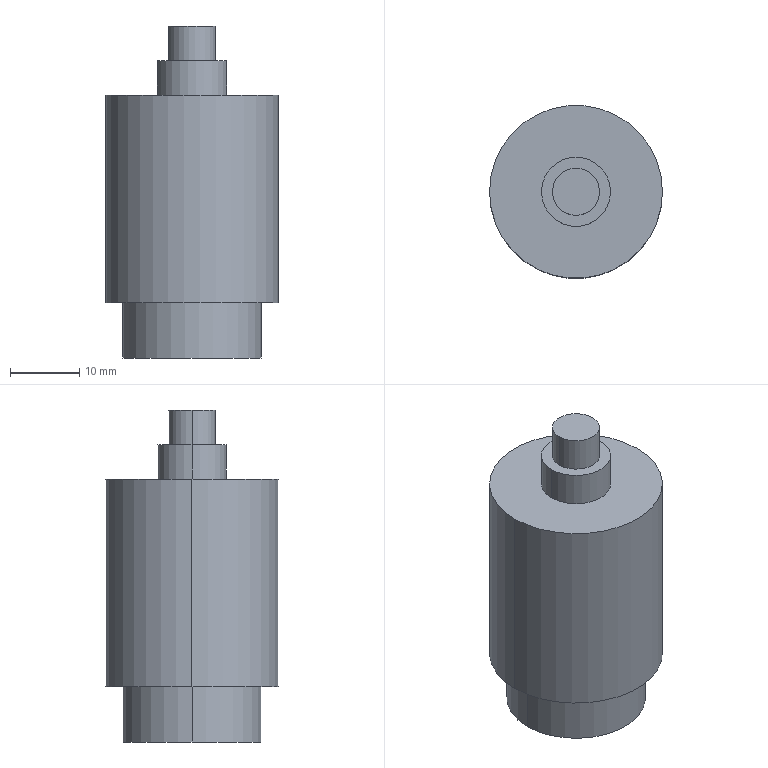Part | SolidWorks | features ICE 3, Extrusion 1 | 1 solid | 13 faces | box 25 x 25 x 48 mm | volume 17814 mm3 | cylinder 8 | plane 5 | commonest cylinder face diameters 6.8 x2 10 x2 20 x2 25 x2
STEP:
#1=CARTESIAN_POINT('',(-10.,0.,-38.));
#2=VERTEX_POINT('',#1);
#3=CARTESIAN_POINT('',(10.,0.,-38.));
#4=VERTEX_POINT('',#3);
#5=CARTESIAN_POINT('',(0.,0.,-38.));
#6=DIRECTION('',(0.,0.,-1.));
#7=DIRECTION('',(-1.,0.,0.));
#8=AXIS2_PLACEMENT_3D('',#5,#6,#7);
#9=CIRCLE('',#8,10.);
#10=EDGE_CURVE('',#2,#4,#9,.T.);
#11=ORIENTED_EDGE('',*,*,#10,.F.);
#12=CARTESIAN_POINT('',(-10.,0.,-30.));
#13=VERTEX_POINT('',#12);
#14=CARTESIAN_POINT('',(-10.,0.,-38.));
#15=DIRECTION('',(0.,0.,1.));
#16=VECTOR('',#15,1000.);
#17=LINE('',#14,#16);
#18=EDGE_CURVE('',#2,#13,#17,.T.);
#19=ORIENTED_EDGE('',*,*,#18,.T.);
#20=CARTESIAN_POINT('',(10.,0.,-30.));
#21=VERTEX_POINT('',#20);
#22=CARTESIAN_POINT('',(0.,0.,-30.));
#23=DIRECTION('',(0.,0.,-1.));
#24=DIRECTION('',(-1.,0.,0.));
#25=AXIS2_PLACEMENT_3D('',#22,#23,#24);
#26=CIRCLE('',#25,10.);
#27=EDGE_CURVE('',#13,#21,#26,.T.);
#28=ORIENTED_EDGE('',*,*,#27,.T.);
#29=CARTESIAN_POINT('',(10.,0.,-38.));
#30=DIRECTION('',(0.,0.,1.));
#31=VECTOR('',#30,1000.);
#32=LINE('',#29,#31);
#33=EDGE_CURVE('',#4,#21,#32,.T.);
#34=ORIENTED_EDGE('',*,*,#33,.F.);
#35=EDGE_LOOP('',(#11,#19,#28,#34));
#36=FACE_OUTER_BOUND('',#35,.T.);
#37=CARTESIAN_POINT('',(0.,0.,-38.));
#38=DIRECTION('',(0.,0.,1.));
#39=DIRECTION('',(1.,0.,0.));
#40=AXIS2_PLACEMENT_3D('',#37,#38,#39);
#41=CYLINDRICAL_SURFACE('',#40,10.);
#42=ADVANCED_FACE('',(#36),#41,.T.);
#43=CARTESIAN_POINT('',(-12.5,0.,-30.));
#44=VERTEX_POINT('',#43);
#45=CARTESIAN_POINT('',(12.5,0.,-30.));
#46=VERTEX_POINT('',#45);
#47=CARTESIAN_POINT('',(0.,0.,-30.));
#48=DIRECTION('',(0.,0.,-1.));
#49=DIRECTION('',(-1.,0.,0.));
#50=AXIS2_PLACEMENT_3D('',#47,#48,#49);
#51=CIRCLE('',#50,12.5);
#52=EDGE_CURVE('',#44,#46,#51,.T.);
#53=ORIENTED_EDGE('',*,*,#52,.F.);
#54=CARTESIAN_POINT('',(-12.5,0.,0.));
#55=VERTEX_POINT('',#54);
#56=CARTESIAN_POINT('',(-12.5,0.,-30.));
#57=DIRECTION('',(0.,0.,1.));
#58=VECTOR('',#57,1000.);
#59=LINE('',#56,#58);
#60=EDGE_CURVE('',#44,#55,#59,.T.);
#61=ORIENTED_EDGE('',*,*,#60,.T.);
#62=CARTESIAN_POINT('',(12.5,0.,0.));
#63=VERTEX_POINT('',#62);
#64=CARTESIAN_POINT('',(0.,0.,0.));
#65=DIRECTION('',(0.,0.,-1.));
#66=DIRECTION('',(-1.,0.,0.));
#67=AXIS2_PLACEMENT_3D('',#64,#65,#66);
#68=CIRCLE('',#67,12.5);
#69=EDGE_CURVE('',#55,#63,#68,.T.);
#70=ORIENTED_EDGE('',*,*,#69,.T.);
#71=CARTESIAN_POINT('',(12.5,0.,-30.));
#72=DIRECTION('',(0.,0.,1.));
#73=VECTOR('',#72,1000.);
#74=LINE('',#71,#73);
#75=EDGE_CURVE('',#46,#63,#74,.T.);
#76=ORIENTED_EDGE('',*,*,#75,.F.);
#77=EDGE_LOOP('',(#53,#61,#70,#76));
#78=FACE_OUTER_BOUND('',#77,.T.);
#79=CARTESIAN_POINT('',(0.,0.,-30.));
#80=DIRECTION('',(0.,0.,1.));
#81=DIRECTION('',(1.,0.,0.));
#82=AXIS2_PLACEMENT_3D('',#79,#80,#81);
#83=CYLINDRICAL_SURFACE('',#82,12.5);
#84=ADVANCED_FACE('',(#78),#83,.T.);
#85=CARTESIAN_POINT('',(3.4,0.,10.));
#86=VERTEX_POINT('',#85);
#87=CARTESIAN_POINT('',(-3.4,0.,10.));
#88=VERTEX_POINT('',#87);
#89=CARTESIAN_POINT('',(0.,0.,10.));
#90=DIRECTION('',(0.,0.,1.));
#91=DIRECTION('',(1.,0.,0.));
#92=AXIS2_PLACEMENT_3D('',#89,#90,#91);
#93=CIRCLE('',#92,3.4);
#94=EDGE_CURVE('',#86,#88,#93,.T.);
#95=ORIENTED_EDGE('',*,*,#94,.F.);
#96=CARTESIAN_POINT('',(3.4,0.,5.));
#97=VERTEX_POINT('',#96);
#98=CARTESIAN_POINT('',(3.4,0.,10.));
#99=DIRECTION('',(0.,0.,-1.));
#100=VECTOR('',#99,1000.);
#101=LINE('',#98,#100);
#102=EDGE_CURVE('',#86,#97,#101,.T.);
#103=ORIENTED_EDGE('',*,*,#102,.T.);
#104=CARTESIAN_POINT('',(-3.4,0.,5.));
#105=VERTEX_POINT('',#104);
#106=CARTESIAN_POINT('',(0.,0.,5.));
#107=DIRECTION('',(0.,0.,1.));
#108=DIRECTION('',(1.,0.,0.));
#109=AXIS2_PLACEMENT_3D('',#106,#107,#108);
#110=CIRCLE('',#109,3.4);
#111=EDGE_CURVE('',#97,#105,#110,.T.);
#112=ORIENTED_EDGE('',*,*,#111,.T.);
#113=CARTESIAN_POINT('',(-3.4,0.,10.));
#114=DIRECTION('',(0.,0.,-1.));
#115=VECTOR('',#114,1000.);
#116=LINE('',#113,#115);
#117=EDGE_CURVE('',#88,#105,#116,.T.);
#118=ORIENTED_EDGE('',*,*,#117,.F.);
#119=EDGE_LOOP('',(#95,#103,#112,#118));
#120=FACE_OUTER_BOUND('',#119,.T.);
#121=CARTESIAN_POINT('',(0.,0.,10.));
#122=DIRECTION('',(0.,0.,-1.));
#123=DIRECTION('',(-1.,0.,0.));
#124=AXIS2_PLACEMENT_3D('',#121,#122,#123);
#125=CYLINDRICAL_SURFACE('',#124,3.4);
#126=ADVANCED_FACE('',(#120),#125,.T.);
#127=CARTESIAN_POINT('',(5.,0.,5.));
#128=VERTEX_POINT('',#127);
#129=CARTESIAN_POINT('',(-5.,0.,5.));
#130=VERTEX_POINT('',#129);
#131=CARTESIAN_POINT('',(0.,0.,5.));
#132=DIRECTION('',(0.,0.,1.));
#133=DIRECTION('',(1.,0.,0.));
#134=AXIS2_PLACEMENT_3D('',#131,#132,#133);
#135=CIRCLE('',#134,5.);
#136=EDGE_CURVE('',#128,#130,#135,.T.);
#137=ORIENTED_EDGE('',*,*,#136,.F.);
#138=CARTESIAN_POINT('',(5.,0.,0.));
#139=VERTEX_POINT('',#138);
#140=CARTESIAN_POINT('',(5.,0.,5.));
#141=DIRECTION('',(0.,0.,-1.));
#142=VECTOR('',#141,1000.);
#143=LINE('',#140,#142);
#144=EDGE_CURVE('',#128,#139,#143,.T.);
#145=ORIENTED_EDGE('',*,*,#144,.T.);
#146=CARTESIAN_POINT('',(-5.,0.,0.));
#147=VERTEX_POINT('',#146);
#148=CARTESIAN_POINT('',(0.,0.,0.));
#149=DIRECTION('',(0.,0.,-1.));
#150=DIRECTION('',(-1.,0.,0.));
#151=AXIS2_PLACEMENT_3D('',#148,#149,#150);
#152=CIRCLE('',#151,5.);
#153=EDGE_CURVE('',#147,#139,#152,.T.);
#154=ORIENTED_EDGE('',*,*,#153,.F.);
#155=CARTESIAN_POINT('',(-5.,0.,5.));
#156=DIRECTION('',(0.,0.,-1.));
#157=VECTOR('',#156,1000.);
#158=LINE('',#155,#157);
#159=EDGE_CURVE('',#130,#147,#158,.T.);
#160=ORIENTED_EDGE('',*,*,#159,.F.);
#161=EDGE_LOOP('',(#137,#145,#154,#160));
#162=FACE_OUTER_BOUND('',#161,.T.);
#163=CARTESIAN_POINT('',(0.,0.,5.));
#164=DIRECTION('',(0.,0.,-1.));
#165=DIRECTION('',(-1.,0.,0.));
#166=AXIS2_PLACEMENT_3D('',#163,#164,#165);
#167=CYLINDRICAL_SURFACE('',#166,5.);
#168=ADVANCED_FACE('',(#162),#167,.T.);
#169=CARTESIAN_POINT('',(0.,0.,-30.));
#170=DIRECTION('',(0.,0.,-1.));
#171=DIRECTION('',(-1.,0.,0.));
#172=AXIS2_PLACEMENT_3D('',#169,#170,#171);
#173=CIRCLE('',#172,12.5);
#174=EDGE_CURVE('',#46,#44,#173,.T.);
#175=ORIENTED_EDGE('',*,*,#174,.T.);
#176=ORIENTED_EDGE('',*,*,#52,.T.);
#177=EDGE_LOOP('',(#175,#176));
#178=FACE_OUTER_BOUND('',#177,.T.);
#179=CARTESIAN_POINT('',(0.,0.,-30.));
#180=DIRECTION('',(0.,0.,-1.));
#181=DIRECTION('',(-1.,0.,0.));
#182=AXIS2_PLACEMENT_3D('',#179,#180,#181);
#183=CIRCLE('',#182,10.);
#184=EDGE_CURVE('',#21,#13,#183,.T.);
#185=ORIENTED_EDGE('',*,*,#184,.F.);
#186=ORIENTED_EDGE('',*,*,#27,.F.);
#187=EDGE_LOOP('',(#185,#186));
#188=FACE_BOUND('',#187,.T.);
#189=CARTESIAN_POINT('',(0.,0.,-30.));
#190=DIRECTION('',(0.,0.,-1.));
#191=DIRECTION('',(-1.,0.,0.));
#192=AXIS2_PLACEMENT_3D('',#189,#190,#191);
#193=PLANE('',#192);
#194=ADVANCED_FACE('',(#178,#188),#193,.T.);
#195=CARTESIAN_POINT('',(0.,0.,5.));
#196=DIRECTION('',(0.,0.,1.));
#197=DIRECTION('',(1.,0.,0.));
#198=AXIS2_PLACEMENT_3D('',#195,#196,#197);
#199=CIRCLE('',#198,5.);
#200=EDGE_CURVE('',#130,#128,#199,.T.);
#201=ORIENTED_EDGE('',*,*,#200,.T.);
#202=ORIENTED_EDGE('',*,*,#136,.T.);
#203=EDGE_LOOP('',(#201,#202));
#204=FACE_OUTER_BOUND('',#203,.T.);
#205=CARTESIAN_POINT('',(0.,0.,5.));
#206=DIRECTION('',(0.,0.,1.));
#207=DIRECTION('',(1.,0.,0.));
#208=AXIS2_PLACEMENT_3D('',#205,#206,#207);
#209=CIRCLE('',#208,3.4);
#210=EDGE_CURVE('',#105,#97,#209,.T.);
#211=ORIENTED_EDGE('',*,*,#210,.F.);
#212=ORIENTED_EDGE('',*,*,#111,.F.);
#213=EDGE_LOOP('',(#211,#212));
#214=FACE_BOUND('',#213,.T.);
#215=CARTESIAN_POINT('',(0.,0.,5.));
#216=DIRECTION('',(0.,0.,1.));
#217=DIRECTION('',(1.,0.,0.));
#218=AXIS2_PLACEMENT_3D('',#215,#216,#217);
#219=PLANE('',#218);
#220=ADVANCED_FACE('',(#204,#214),#219,.T.);
#221=ORIENTED_EDGE('',*,*,#144,.F.);
#222=ORIENTED_EDGE('',*,*,#200,.F.);
#223=ORIENTED_EDGE('',*,*,#159,.T.);
#224=CARTESIAN_POINT('',(0.,0.,0.));
#225=DIRECTION('',(0.,0.,-1.));
#226=DIRECTION('',(-1.,0.,0.));
#227=AXIS2_PLACEMENT_3D('',#224,#225,#226);
#228=CIRCLE('',#227,5.);
#229=EDGE_CURVE('',#139,#147,#228,.T.);
#230=ORIENTED_EDGE('',*,*,#229,.F.);
#231=EDGE_LOOP('',(#221,#222,#223,#230));
#232=FACE_OUTER_BOUND('',#231,.T.);
#233=CARTESIAN_POINT('',(0.,0.,5.));
#234=DIRECTION('',(0.,0.,-1.));
#235=DIRECTION('',(-1.,0.,0.));
#236=AXIS2_PLACEMENT_3D('',#233,#234,#235);
#237=CYLINDRICAL_SURFACE('',#236,5.);
#238=ADVANCED_FACE('',(#232),#237,.T.);
#239=ORIENTED_EDGE('',*,*,#102,.F.);
#240=CARTESIAN_POINT('',(0.,0.,10.));
#241=DIRECTION('',(0.,0.,1.));
#242=DIRECTION('',(1.,0.,0.));
#243=AXIS2_PLACEMENT_3D('',#240,#241,#242);
#244=CIRCLE('',#243,3.4);
#245=EDGE_CURVE('',#88,#86,#244,.T.);
#246=ORIENTED_EDGE('',*,*,#245,.F.);
#247=ORIENTED_EDGE('',*,*,#117,.T.);
#248=ORIENTED_EDGE('',*,*,#210,.T.);
#249=EDGE_LOOP('',(#239,#246,#247,#248));
#250=FACE_OUTER_BOUND('',#249,.T.);
#251=CARTESIAN_POINT('',(0.,0.,10.));
#252=DIRECTION('',(0.,0.,-1.));
#253=DIRECTION('',(-1.,0.,0.));
#254=AXIS2_PLACEMENT_3D('',#251,#252,#253);
#255=CYLINDRICAL_SURFACE('',#254,3.4);
#256=ADVANCED_FACE('',(#250),#255,.T.);
#257=ORIENTED_EDGE('',*,*,#245,.T.);
#258=ORIENTED_EDGE('',*,*,#94,.T.);
#259=EDGE_LOOP('',(#257,#258));
#260=FACE_OUTER_BOUND('',#259,.T.);
#261=CARTESIAN_POINT('',(0.,0.,10.));
#262=DIRECTION('',(0.,0.,1.));
#263=DIRECTION('',(1.,0.,0.));
#264=AXIS2_PLACEMENT_3D('',#261,#262,#263);
#265=PLANE('',#264);
#266=ADVANCED_FACE('',(#260),#265,.T.);
#267=CARTESIAN_POINT('',(0.,0.,0.));
#268=DIRECTION('',(0.,0.,-1.));
#269=DIRECTION('',(-1.,0.,0.));
#270=AXIS2_PLACEMENT_3D('',#267,#268,#269);
#271=CIRCLE('',#270,12.5);
#272=EDGE_CURVE('',#63,#55,#271,.T.);
#273=ORIENTED_EDGE('',*,*,#272,.F.);
#274=ORIENTED_EDGE('',*,*,#69,.F.);
#275=EDGE_LOOP('',(#273,#274));
#276=FACE_OUTER_BOUND('',#275,.T.);
#277=ORIENTED_EDGE('',*,*,#153,.T.);
#278=ORIENTED_EDGE('',*,*,#229,.T.);
#279=EDGE_LOOP('',(#277,#278));
#280=FACE_BOUND('',#279,.T.);
#281=CARTESIAN_POINT('',(0.,0.,0.));
#282=DIRECTION('',(0.,0.,-1.));
#283=DIRECTION('',(-1.,0.,0.));
#284=AXIS2_PLACEMENT_3D('',#281,#282,#283);
#285=PLANE('',#284);
#286=ADVANCED_FACE('',(#276,#280),#285,.F.);
#287=ORIENTED_EDGE('',*,*,#60,.F.);
#288=ORIENTED_EDGE('',*,*,#174,.F.);
#289=ORIENTED_EDGE('',*,*,#75,.T.);
#290=ORIENTED_EDGE('',*,*,#272,.T.);
#291=EDGE_LOOP('',(#287,#288,#289,#290));
#292=FACE_OUTER_BOUND('',#291,.T.);
#293=CARTESIAN_POINT('',(0.,0.,-30.));
#294=DIRECTION('',(0.,0.,1.));
#295=DIRECTION('',(1.,0.,0.));
#296=AXIS2_PLACEMENT_3D('',#293,#294,#295);
#297=CYLINDRICAL_SURFACE('',#296,12.5);
#298=ADVANCED_FACE('',(#292),#297,.T.);
#299=ORIENTED_EDGE('',*,*,#18,.F.);
#300=CARTESIAN_POINT('',(0.,0.,-38.));
#301=DIRECTION('',(0.,0.,-1.));
#302=DIRECTION('',(-1.,0.,0.));
#303=AXIS2_PLACEMENT_3D('',#300,#301,#302);
#304=CIRCLE('',#303,10.);
#305=EDGE_CURVE('',#4,#2,#304,.T.);
#306=ORIENTED_EDGE('',*,*,#305,.F.);
#307=ORIENTED_EDGE('',*,*,#33,.T.);
#308=ORIENTED_EDGE('',*,*,#184,.T.);
#309=EDGE_LOOP('',(#299,#306,#307,#308));
#310=FACE_OUTER_BOUND('',#309,.T.);
#311=CARTESIAN_POINT('',(0.,0.,-38.));
#312=DIRECTION('',(0.,0.,1.));
#313=DIRECTION('',(1.,0.,0.));
#314=AXIS2_PLACEMENT_3D('',#311,#312,#313);
#315=CYLINDRICAL_SURFACE('',#314,10.);
#316=ADVANCED_FACE('',(#310),#315,.T.);
#317=ORIENTED_EDGE('',*,*,#305,.T.);
#318=ORIENTED_EDGE('',*,*,#10,.T.);
#319=EDGE_LOOP('',(#317,#318));
#320=FACE_OUTER_BOUND('',#319,.T.);
#321=CARTESIAN_POINT('',(0.,0.,-38.));
#322=DIRECTION('',(0.,0.,-1.));
#323=DIRECTION('',(-1.,0.,0.));
#324=AXIS2_PLACEMENT_3D('',#321,#322,#323);
#325=PLANE('',#324);
#326=ADVANCED_FACE('',(#320),#325,.T.);
#327=CLOSED_SHELL('',(#42,#84,#126,#168,#194,#220,#238,#256,#266,#286,#298,#316,#326));
#328=MANIFOLD_SOLID_BREP('',#327);
#329=CARTESIAN_POINT('',(0.,0.,0.));
#330=DIRECTION('',(0.,0.,1.));
#331=DIRECTION('',(1.,0.,0.));
#332=AXIS2_PLACEMENT_3D('',#329,#330,#331);
#333=(LENGTH_UNIT()NAMED_UNIT(*)SI_UNIT(.MILLI.,.METRE.));
#334=UNCERTAINTY_MEASURE_WITH_UNIT(LENGTH_MEASURE(0.00001),#333,'','');
#335=(NAMED_UNIT(*)PLANE_ANGLE_UNIT()SI_UNIT($,.RADIAN.));
#336=(NAMED_UNIT(*)SI_UNIT($,.STERADIAN.)SOLID_ANGLE_UNIT());
#337=(GEOMETRIC_REPRESENTATION_CONTEXT(3)GLOBAL_UNCERTAINTY_ASSIGNED_CONTEXT((#334))GLOBAL_UNIT_ASSIGNED_CONTEXT((#333,#335,#336))REPRESENTATION_CONTEXT('',''));
#338=ADVANCED_BREP_SHAPE_REPRESENTATION('',(#328,#332),#337);